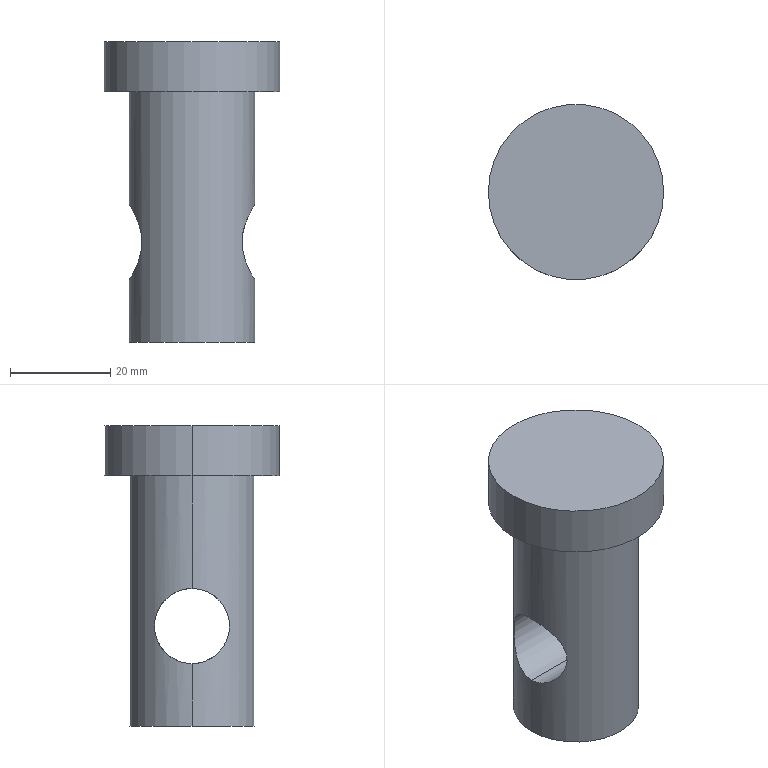Part | SolidWorks | features ICE 2, Chamfer 1, Extrusion 1 | 1 solid | 9 faces | box 35 x 35 x 60 mm | volume 29956 mm3 | cylinder 6 | plane 3 | commonest cylinder face diameters 15 x2 25 x2 35 x2
STEP:
#1=CARTESIAN_POINT('',(-12.5,0.,27.5));
#2=VERTEX_POINT('',#1);
#3=CARTESIAN_POINT('',(-12.5,0.,12.5));
#4=VERTEX_POINT('',#3);
#5=CARTESIAN_POINT('',(-12.5,0.,27.5));
#6=CARTESIAN_POINT('',(-12.5,-0.5065,27.5));
#7=CARTESIAN_POINT('',(-12.469,-1.005,27.449));
#8=CARTESIAN_POINT('',(-12.381,-1.74,27.3));
#9=CARTESIAN_POINT('',(-12.344,-1.984,27.237));
#10=CARTESIAN_POINT('',(-12.258,-2.461,27.089));
#11=CARTESIAN_POINT('',(-12.209,-2.693,27.004));
#12=CARTESIAN_POINT('',(-12.1,-3.145,26.813));
#13=CARTESIAN_POINT('',(-12.041,-3.365,26.707));
#14=CARTESIAN_POINT('',(-11.912,-3.794,26.474));
#15=CARTESIAN_POINT('',(-11.843,-4.004,26.347));
#16=CARTESIAN_POINT('',(-11.628,-4.606,25.939));
#17=CARTESIAN_POINT('',(-11.474,-4.974,25.633));
#18=CARTESIAN_POINT('',(-11.157,-5.65,24.956));
#19=CARTESIAN_POINT('',(-10.993,-5.957,24.581));
#20=CARTESIAN_POINT('',(-10.687,-6.49,23.788));
#21=CARTESIAN_POINT('',(-10.543,-6.72,23.367));
#22=CARTESIAN_POINT('',(-10.354,-7.005,22.691));
#23=CARTESIAN_POINT('',(-10.295,-7.09,22.458));
#24=CARTESIAN_POINT('',(-10.193,-7.237,21.985));
#25=CARTESIAN_POINT('',(-10.148,-7.298,21.745));
#26=CARTESIAN_POINT('',(-10.076,-7.398,21.258));
#27=CARTESIAN_POINT('',(-10.048,-7.436,21.011));
#28=CARTESIAN_POINT('',(-10.01,-7.487,20.509));
#29=CARTESIAN_POINT('',(-10.,-7.5,20.253));
#30=CARTESIAN_POINT('',(-10.,-7.5,19.498));
#31=CARTESIAN_POINT('',(-10.038,-7.45,19.));
#32=CARTESIAN_POINT('',(-10.147,-7.3,18.261));
#33=CARTESIAN_POINT('',(-10.192,-7.238,18.019));
#34=CARTESIAN_POINT('',(-10.294,-7.092,17.547));
#35=CARTESIAN_POINT('',(-10.352,-7.008,17.316));
#36=CARTESIAN_POINT('',(-10.54,-6.724,16.641));
#37=CARTESIAN_POINT('',(-10.688,-6.49,16.21));
#38=CARTESIAN_POINT('',(-10.995,-5.954,15.414));
#39=CARTESIAN_POINT('',(-11.156,-5.651,15.045));
#40=CARTESIAN_POINT('',(-11.476,-4.97,14.362));
#41=CARTESIAN_POINT('',(-11.63,-4.601,14.057));
#42=CARTESIAN_POINT('',(-11.843,-4.004,13.654));
#43=CARTESIAN_POINT('',(-11.911,-3.798,13.528));
#44=CARTESIAN_POINT('',(-12.039,-3.369,13.295));
#45=CARTESIAN_POINT('',(-12.1,-3.146,13.187));
#46=CARTESIAN_POINT('',(-12.264,-2.463,12.899));
#47=CARTESIAN_POINT('',(-12.35,-1.993,12.752));
#48=CARTESIAN_POINT('',(-12.439,-1.262,12.603));
#49=CARTESIAN_POINT('',(-12.461,-1.014,12.565));
#50=CARTESIAN_POINT('',(-12.492,-0.5103,12.513));
#51=CARTESIAN_POINT('',(-12.5,-0.2541,12.5));
#52=CARTESIAN_POINT('',(-12.5,0.,12.5));
#53=B_SPLINE_CURVE_WITH_KNOTS('',3,(#5,#6,#7,#8,#9,#10,#11,#12,#13,#14,#15,#16,#17,#18,#19,#20,#21,#22,#23,#24,#25,#26,#27,#28,#29,#30,#31,#32,#33,#34,#35,#36,#37,#38,#39,#40,#41,#42,#43,#44,#45,#46,#47,#48,#49,#50,#51,#52),.UNSPECIFIED.,.F.,.F.,(4,2,2,2,2,2,2,2,2,2,2,2,2,2,2,2,2,2,2,2,2,2,2,4),(0.02406,0.02556,0.02631,0.02706,0.02781,0.02856,0.03007,0.03157,0.03307,0.03382,0.03457,0.03532,0.03607,0.03757,0.03832,0.03907,0.04057,0.04207,0.04357,0.04432,0.04507,0.04658,0.04733,0.04808),.UNSPECIFIED.);
#54=EDGE_CURVE('',#2,#4,#53,.T.);
#55=ORIENTED_EDGE('',*,*,#54,.F.);
#56=CARTESIAN_POINT('',(12.5,0.,27.5));
#57=VERTEX_POINT('',#56);
#58=CARTESIAN_POINT('',(-30.,0.,27.5));
#59=DIRECTION('',(1.,0.,0.));
#60=VECTOR('',#59,1000.);
#61=LINE('',#58,#60);
#62=EDGE_CURVE('',#2,#57,#61,.T.);
#63=ORIENTED_EDGE('',*,*,#62,.T.);
#64=CARTESIAN_POINT('',(12.5,0.,12.5));
#65=VERTEX_POINT('',#64);
#66=CARTESIAN_POINT('',(12.5,0.,12.5));
#67=CARTESIAN_POINT('',(12.5,-0.5093,12.5));
#68=CARTESIAN_POINT('',(12.469,-1.008,12.551));
#69=CARTESIAN_POINT('',(12.351,-1.985,12.75));
#70=CARTESIAN_POINT('',(12.263,-2.468,12.901));
#71=CARTESIAN_POINT('',(12.045,-3.373,13.283));
#72=CARTESIAN_POINT('',(11.916,-3.8,13.516));
#73=CARTESIAN_POINT('',(11.628,-4.606,14.061));
#74=CARTESIAN_POINT('',(11.473,-4.976,14.368));
#75=CARTESIAN_POINT('',(11.236,-5.481,14.875));
#76=CARTESIAN_POINT('',(11.156,-5.641,15.052));
#77=CARTESIAN_POINT('',(10.996,-5.946,15.423));
#78=CARTESIAN_POINT('',(10.917,-6.091,15.617));
#79=CARTESIAN_POINT('',(10.686,-6.492,16.214));
#80=CARTESIAN_POINT('',(10.542,-6.721,16.636));
#81=CARTESIAN_POINT('',(10.291,-7.099,17.531));
#82=CARTESIAN_POINT('',(10.184,-7.249,18.011));
#83=CARTESIAN_POINT('',(10.076,-7.398,18.743));
#84=CARTESIAN_POINT('',(10.048,-7.436,18.989));
#85=CARTESIAN_POINT('',(10.01,-7.487,19.489));
#86=CARTESIAN_POINT('',(10.,-7.5,19.743));
#87=CARTESIAN_POINT('',(10.,-7.5,20.505));
#88=CARTESIAN_POINT('',(10.039,-7.449,21.004));
#89=CARTESIAN_POINT('',(10.147,-7.3,21.738));
#90=CARTESIAN_POINT('',(10.192,-7.238,21.982));
#91=CARTESIAN_POINT('',(10.294,-7.091,22.456));
#92=CARTESIAN_POINT('',(10.352,-7.007,22.686));
#93=CARTESIAN_POINT('',(10.478,-6.817,23.136));
#94=CARTESIAN_POINT('',(10.546,-6.712,23.355));
#95=CARTESIAN_POINT('',(10.69,-6.481,23.782));
#96=CARTESIAN_POINT('',(10.765,-6.355,23.991));
#97=CARTESIAN_POINT('',(10.997,-5.952,24.589));
#98=CARTESIAN_POINT('',(11.157,-5.649,24.957));
#99=CARTESIAN_POINT('',(11.396,-5.141,25.467));
#100=CARTESIAN_POINT('',(11.475,-4.961,25.63));
#101=CARTESIAN_POINT('',(11.629,-4.59,25.936));
#102=CARTESIAN_POINT('',(11.703,-4.397,26.08));
#103=CARTESIAN_POINT('',(11.916,-3.8,26.484));
#104=CARTESIAN_POINT('',(12.045,-3.375,26.716));
#105=CARTESIAN_POINT('',(12.209,-2.691,27.005));
#106=CARTESIAN_POINT('',(12.259,-2.456,27.091));
#107=CARTESIAN_POINT('',(12.344,-1.982,27.238));
#108=CARTESIAN_POINT('',(12.38,-1.742,27.299));
#109=CARTESIAN_POINT('',(12.439,-1.255,27.398));
#110=CARTESIAN_POINT('',(12.462,-1.009,27.436));
#111=CARTESIAN_POINT('',(12.492,-0.5089,27.487));
#112=CARTESIAN_POINT('',(12.5,-0.2538,27.5));
#113=CARTESIAN_POINT('',(12.5,0.,27.5));
#114=B_SPLINE_CURVE_WITH_KNOTS('',3,(#66,#67,#68,#69,#70,#71,#72,#73,#74,#75,#76,#77,#78,#79,#80,#81,#82,#83,#84,#85,#86,#87,#88,#89,#90,#91,#92,#93,#94,#95,#96,#97,#98,#99,#100,#101,#102,#103,#104,#105,#106,#107,#108,#109,#110,#111,#112,#113),.UNSPECIFIED.,.F.,.F.,(4,2,2,2,2,2,2,2,2,2,2,2,2,2,2,2,2,2,2,2,2,2,2,4),(0.,0.001504,0.003008,0.004512,0.006015,0.006767,0.007519,0.009023,0.01053,0.01128,0.01203,0.01353,0.01429,0.01504,0.01579,0.01654,0.01805,0.0188,0.01955,0.02105,0.02181,0.02256,0.02331,0.02406),.UNSPECIFIED.);
#115=EDGE_CURVE('',#65,#57,#114,.T.);
#116=ORIENTED_EDGE('',*,*,#115,.F.);
#117=CARTESIAN_POINT('',(-30.,0.,12.5));
#118=DIRECTION('',(1.,0.,0.));
#119=VECTOR('',#118,1000.);
#120=LINE('',#117,#119);
#121=EDGE_CURVE('',#4,#65,#120,.T.);
#122=ORIENTED_EDGE('',*,*,#121,.F.);
#123=EDGE_LOOP('',(#55,#63,#116,#122));
#124=FACE_OUTER_BOUND('',#123,.T.);
#125=CARTESIAN_POINT('',(-30.,0.,20.));
#126=DIRECTION('',(1.,0.,0.));
#127=DIRECTION('',(0.,0.,-1.));
#128=AXIS2_PLACEMENT_3D('',#125,#126,#127);
#129=CYLINDRICAL_SURFACE('',#128,7.5);
#130=ADVANCED_FACE('',(#124),#129,.F.);
#131=CARTESIAN_POINT('',(-12.5,0.,50.));
#132=VERTEX_POINT('',#131);
#133=CARTESIAN_POINT('',(12.5,0.,50.));
#134=VERTEX_POINT('',#133);
#135=CARTESIAN_POINT('',(0.,0.,50.));
#136=DIRECTION('',(0.,0.,-1.));
#137=DIRECTION('',(-1.,0.,0.));
#138=AXIS2_PLACEMENT_3D('',#135,#136,#137);
#139=CIRCLE('',#138,12.5);
#140=EDGE_CURVE('',#132,#134,#139,.T.);
#141=ORIENTED_EDGE('',*,*,#140,.T.);
#142=CARTESIAN_POINT('',(12.5,0.,50.));
#143=DIRECTION('',(0.,0.,-1.));
#144=VECTOR('',#143,1000.);
#145=LINE('',#142,#144);
#146=EDGE_CURVE('',#134,#57,#145,.T.);
#147=ORIENTED_EDGE('',*,*,#146,.T.);
#148=CARTESIAN_POINT('',(12.5,0.,27.5));
#149=CARTESIAN_POINT('',(12.5,0.5065,27.5));
#150=CARTESIAN_POINT('',(12.469,1.005,27.449));
#151=CARTESIAN_POINT('',(12.381,1.74,27.3));
#152=CARTESIAN_POINT('',(12.344,1.984,27.237));
#153=CARTESIAN_POINT('',(12.258,2.461,27.089));
#154=CARTESIAN_POINT('',(12.209,2.693,27.004));
#155=CARTESIAN_POINT('',(12.1,3.145,26.813));
#156=CARTESIAN_POINT('',(12.041,3.365,26.707));
#157=CARTESIAN_POINT('',(11.912,3.794,26.474));
#158=CARTESIAN_POINT('',(11.843,4.004,26.347));
#159=CARTESIAN_POINT('',(11.628,4.606,25.939));
#160=CARTESIAN_POINT('',(11.474,4.974,25.633));
#161=CARTESIAN_POINT('',(11.157,5.65,24.956));
#162=CARTESIAN_POINT('',(10.993,5.957,24.581));
#163=CARTESIAN_POINT('',(10.687,6.49,23.788));
#164=CARTESIAN_POINT('',(10.543,6.72,23.367));
#165=CARTESIAN_POINT('',(10.354,7.005,22.691));
#166=CARTESIAN_POINT('',(10.295,7.09,22.458));
#167=CARTESIAN_POINT('',(10.193,7.237,21.985));
#168=CARTESIAN_POINT('',(10.148,7.298,21.745));
#169=CARTESIAN_POINT('',(10.076,7.398,21.258));
#170=CARTESIAN_POINT('',(10.048,7.436,21.011));
#171=CARTESIAN_POINT('',(10.01,7.487,20.509));
#172=CARTESIAN_POINT('',(10.,7.5,20.253));
#173=CARTESIAN_POINT('',(10.,7.5,19.498));
#174=CARTESIAN_POINT('',(10.038,7.45,19.));
#175=CARTESIAN_POINT('',(10.147,7.3,18.261));
#176=CARTESIAN_POINT('',(10.192,7.238,18.019));
#177=CARTESIAN_POINT('',(10.294,7.092,17.547));
#178=CARTESIAN_POINT('',(10.352,7.008,17.316));
#179=CARTESIAN_POINT('',(10.54,6.724,16.641));
#180=CARTESIAN_POINT('',(10.688,6.49,16.21));
#181=CARTESIAN_POINT('',(10.995,5.954,15.414));
#182=CARTESIAN_POINT('',(11.156,5.651,15.045));
#183=CARTESIAN_POINT('',(11.476,4.97,14.362));
#184=CARTESIAN_POINT('',(11.63,4.601,14.057));
#185=CARTESIAN_POINT('',(11.843,4.004,13.654));
#186=CARTESIAN_POINT('',(11.911,3.798,13.528));
#187=CARTESIAN_POINT('',(12.039,3.369,13.295));
#188=CARTESIAN_POINT('',(12.1,3.146,13.187));
#189=CARTESIAN_POINT('',(12.264,2.463,12.899));
#190=CARTESIAN_POINT('',(12.35,1.993,12.752));
#191=CARTESIAN_POINT('',(12.439,1.262,12.603));
#192=CARTESIAN_POINT('',(12.461,1.014,12.565));
#193=CARTESIAN_POINT('',(12.492,0.5103,12.513));
#194=CARTESIAN_POINT('',(12.5,0.2541,12.5));
#195=CARTESIAN_POINT('',(12.5,0.,12.5));
#196=B_SPLINE_CURVE_WITH_KNOTS('',3,(#148,#149,#150,#151,#152,#153,#154,#155,#156,#157,#158,#159,#160,#161,#162,#163,#164,#165,#166,#167,#168,#169,#170,#171,#172,#173,#174,#175,#176,#177,#178,#179,#180,#181,#182,#183,#184,#185,#186,#187,#188,#189,#190,#191,#192,#193,#194,#195),.UNSPECIFIED.,.F.,.F.,(4,2,2,2,2,2,2,2,2,2,2,2,2,2,2,2,2,2,2,2,2,2,2,4),(0.02406,0.02556,0.02631,0.02706,0.02781,0.02856,0.03007,0.03157,0.03307,0.03382,0.03457,0.03532,0.03607,0.03757,0.03832,0.03907,0.04057,0.04207,0.04357,0.04432,0.04507,0.04658,0.04733,0.04808),.UNSPECIFIED.);
#197=EDGE_CURVE('',#57,#65,#196,.T.);
#198=ORIENTED_EDGE('',*,*,#197,.T.);
#199=CARTESIAN_POINT('',(12.5,0.,0.));
#200=VERTEX_POINT('',#199);
#201=CARTESIAN_POINT('',(12.5,0.,50.));
#202=DIRECTION('',(0.,0.,-1.));
#203=VECTOR('',#202,1000.);
#204=LINE('',#201,#203);
#205=EDGE_CURVE('',#65,#200,#204,.T.);
#206=ORIENTED_EDGE('',*,*,#205,.T.);
#207=CARTESIAN_POINT('',(-12.5,0.,0.));
#208=VERTEX_POINT('',#207);
#209=CARTESIAN_POINT('',(0.,0.,0.));
#210=DIRECTION('',(0.,0.,-1.));
#211=DIRECTION('',(-1.,0.,0.));
#212=AXIS2_PLACEMENT_3D('',#209,#210,#211);
#213=CIRCLE('',#212,12.5);
#214=EDGE_CURVE('',#208,#200,#213,.T.);
#215=ORIENTED_EDGE('',*,*,#214,.F.);
#216=CARTESIAN_POINT('',(-12.5,0.,50.));
#217=DIRECTION('',(0.,0.,-1.));
#218=VECTOR('',#217,1000.);
#219=LINE('',#216,#218);
#220=EDGE_CURVE('',#4,#208,#219,.T.);
#221=ORIENTED_EDGE('',*,*,#220,.F.);
#222=CARTESIAN_POINT('',(-12.5,0.,12.5));
#223=CARTESIAN_POINT('',(-12.5,0.5093,12.5));
#224=CARTESIAN_POINT('',(-12.469,1.008,12.551));
#225=CARTESIAN_POINT('',(-12.351,1.985,12.75));
#226=CARTESIAN_POINT('',(-12.263,2.468,12.901));
#227=CARTESIAN_POINT('',(-12.045,3.373,13.283));
#228=CARTESIAN_POINT('',(-11.916,3.8,13.516));
#229=CARTESIAN_POINT('',(-11.628,4.606,14.061));
#230=CARTESIAN_POINT('',(-11.473,4.976,14.368));
#231=CARTESIAN_POINT('',(-11.236,5.481,14.875));
#232=CARTESIAN_POINT('',(-11.156,5.641,15.052));
#233=CARTESIAN_POINT('',(-10.996,5.946,15.423));
#234=CARTESIAN_POINT('',(-10.917,6.091,15.617));
#235=CARTESIAN_POINT('',(-10.686,6.492,16.214));
#236=CARTESIAN_POINT('',(-10.542,6.721,16.636));
#237=CARTESIAN_POINT('',(-10.291,7.099,17.531));
#238=CARTESIAN_POINT('',(-10.184,7.249,18.011));
#239=CARTESIAN_POINT('',(-10.076,7.398,18.743));
#240=CARTESIAN_POINT('',(-10.048,7.436,18.989));
#241=CARTESIAN_POINT('',(-10.01,7.487,19.489));
#242=CARTESIAN_POINT('',(-10.,7.5,19.743));
#243=CARTESIAN_POINT('',(-10.,7.5,20.505));
#244=CARTESIAN_POINT('',(-10.039,7.449,21.004));
#245=CARTESIAN_POINT('',(-10.147,7.3,21.738));
#246=CARTESIAN_POINT('',(-10.192,7.238,21.982));
#247=CARTESIAN_POINT('',(-10.294,7.091,22.456));
#248=CARTESIAN_POINT('',(-10.352,7.007,22.686));
#249=CARTESIAN_POINT('',(-10.478,6.817,23.136));
#250=CARTESIAN_POINT('',(-10.546,6.712,23.355));
#251=CARTESIAN_POINT('',(-10.69,6.481,23.782));
#252=CARTESIAN_POINT('',(-10.765,6.355,23.991));
#253=CARTESIAN_POINT('',(-10.997,5.952,24.589));
#254=CARTESIAN_POINT('',(-11.157,5.649,24.957));
#255=CARTESIAN_POINT('',(-11.396,5.141,25.467));
#256=CARTESIAN_POINT('',(-11.475,4.961,25.63));
#257=CARTESIAN_POINT('',(-11.629,4.59,25.936));
#258=CARTESIAN_POINT('',(-11.703,4.397,26.08));
#259=CARTESIAN_POINT('',(-11.916,3.8,26.484));
#260=CARTESIAN_POINT('',(-12.045,3.375,26.716));
#261=CARTESIAN_POINT('',(-12.209,2.691,27.005));
#262=CARTESIAN_POINT('',(-12.259,2.456,27.091));
#263=CARTESIAN_POINT('',(-12.344,1.982,27.238));
#264=CARTESIAN_POINT('',(-12.38,1.742,27.299));
#265=CARTESIAN_POINT('',(-12.439,1.255,27.398));
#266=CARTESIAN_POINT('',(-12.462,1.009,27.436));
#267=CARTESIAN_POINT('',(-12.492,0.5089,27.487));
#268=CARTESIAN_POINT('',(-12.5,0.2538,27.5));
#269=CARTESIAN_POINT('',(-12.5,0.,27.5));
#270=B_SPLINE_CURVE_WITH_KNOTS('',3,(#222,#223,#224,#225,#226,#227,#228,#229,#230,#231,#232,#233,#234,#235,#236,#237,#238,#239,#240,#241,#242,#243,#244,#245,#246,#247,#248,#249,#250,#251,#252,#253,#254,#255,#256,#257,#258,#259,#260,#261,#262,#263,#264,#265,#266,#267,#268,#269),.UNSPECIFIED.,.F.,.F.,(4,2,2,2,2,2,2,2,2,2,2,2,2,2,2,2,2,2,2,2,2,2,2,4),(0.,0.001504,0.003008,0.004512,0.006015,0.006767,0.007519,0.009023,0.01053,0.01128,0.01203,0.01353,0.01429,0.01504,0.01579,0.01654,0.01805,0.0188,0.01955,0.02105,0.02181,0.02256,0.02331,0.02406),.UNSPECIFIED.);
#271=EDGE_CURVE('',#4,#2,#270,.T.);
#272=ORIENTED_EDGE('',*,*,#271,.T.);
#273=CARTESIAN_POINT('',(-12.5,0.,50.));
#274=DIRECTION('',(0.,0.,-1.));
#275=VECTOR('',#274,1000.);
#276=LINE('',#273,#275);
#277=EDGE_CURVE('',#132,#2,#276,.T.);
#278=ORIENTED_EDGE('',*,*,#277,.F.);
#279=EDGE_LOOP('',(#141,#147,#198,#206,#215,#221,#272,#278));
#280=FACE_OUTER_BOUND('',#279,.T.);
#281=CARTESIAN_POINT('',(0.,0.,50.));
#282=DIRECTION('',(0.,0.,-1.));
#283=DIRECTION('',(-1.,0.,0.));
#284=AXIS2_PLACEMENT_3D('',#281,#282,#283);
#285=CYLINDRICAL_SURFACE('',#284,12.5);
#286=ADVANCED_FACE('',(#280),#285,.T.);
#287=CARTESIAN_POINT('',(17.5,0.,60.));
#288=VERTEX_POINT('',#287);
#289=CARTESIAN_POINT('',(-17.5,0.,60.));
#290=VERTEX_POINT('',#289);
#291=CARTESIAN_POINT('',(0.,0.,60.));
#292=DIRECTION('',(0.,0.,1.));
#293=DIRECTION('',(1.,0.,0.));
#294=AXIS2_PLACEMENT_3D('',#291,#292,#293);
#295=CIRCLE('',#294,17.5);
#296=EDGE_CURVE('',#288,#290,#295,.T.);
#297=ORIENTED_EDGE('',*,*,#296,.F.);
#298=CARTESIAN_POINT('',(17.5,0.,50.));
#299=VERTEX_POINT('',#298);
#300=CARTESIAN_POINT('',(17.5,0.,60.));
#301=DIRECTION('',(0.,0.,-1.));
#302=VECTOR('',#301,1000.);
#303=LINE('',#300,#302);
#304=EDGE_CURVE('',#288,#299,#303,.T.);
#305=ORIENTED_EDGE('',*,*,#304,.T.);
#306=CARTESIAN_POINT('',(-17.5,0.,50.));
#307=VERTEX_POINT('',#306);
#308=CARTESIAN_POINT('',(0.,0.,50.));
#309=DIRECTION('',(0.,0.,-1.));
#310=DIRECTION('',(-1.,0.,0.));
#311=AXIS2_PLACEMENT_3D('',#308,#309,#310);
#312=CIRCLE('',#311,17.5);
#313=EDGE_CURVE('',#307,#299,#312,.T.);
#314=ORIENTED_EDGE('',*,*,#313,.F.);
#315=CARTESIAN_POINT('',(-17.5,0.,60.));
#316=DIRECTION('',(0.,0.,-1.));
#317=VECTOR('',#316,1000.);
#318=LINE('',#315,#317);
#319=EDGE_CURVE('',#290,#307,#318,.T.);
#320=ORIENTED_EDGE('',*,*,#319,.F.);
#321=EDGE_LOOP('',(#297,#305,#314,#320));
#322=FACE_OUTER_BOUND('',#321,.T.);
#323=CARTESIAN_POINT('',(0.,0.,60.));
#324=DIRECTION('',(0.,0.,-1.));
#325=DIRECTION('',(-1.,0.,0.));
#326=AXIS2_PLACEMENT_3D('',#323,#324,#325);
#327=CYLINDRICAL_SURFACE('',#326,17.5);
#328=ADVANCED_FACE('',(#322),#327,.T.);
#329=ORIENTED_EDGE('',*,*,#304,.F.);
#330=CARTESIAN_POINT('',(0.,0.,60.));
#331=DIRECTION('',(0.,0.,1.));
#332=DIRECTION('',(1.,0.,0.));
#333=AXIS2_PLACEMENT_3D('',#330,#331,#332);
#334=CIRCLE('',#333,17.5);
#335=EDGE_CURVE('',#290,#288,#334,.T.);
#336=ORIENTED_EDGE('',*,*,#335,.F.);
#337=ORIENTED_EDGE('',*,*,#319,.T.);
#338=CARTESIAN_POINT('',(0.,0.,50.));
#339=DIRECTION('',(0.,0.,-1.));
#340=DIRECTION('',(-1.,0.,0.));
#341=AXIS2_PLACEMENT_3D('',#338,#339,#340);
#342=CIRCLE('',#341,17.5);
#343=EDGE_CURVE('',#299,#307,#342,.T.);
#344=ORIENTED_EDGE('',*,*,#343,.F.);
#345=EDGE_LOOP('',(#329,#336,#337,#344));
#346=FACE_OUTER_BOUND('',#345,.T.);
#347=CARTESIAN_POINT('',(0.,0.,60.));
#348=DIRECTION('',(0.,0.,-1.));
#349=DIRECTION('',(-1.,0.,0.));
#350=AXIS2_PLACEMENT_3D('',#347,#348,#349);
#351=CYLINDRICAL_SURFACE('',#350,17.5);
#352=ADVANCED_FACE('',(#346),#351,.T.);
#353=ORIENTED_EDGE('',*,*,#335,.T.);
#354=ORIENTED_EDGE('',*,*,#296,.T.);
#355=EDGE_LOOP('',(#353,#354));
#356=FACE_OUTER_BOUND('',#355,.T.);
#357=CARTESIAN_POINT('',(0.,0.,60.));
#358=DIRECTION('',(0.,0.,1.));
#359=DIRECTION('',(1.,0.,0.));
#360=AXIS2_PLACEMENT_3D('',#357,#358,#359);
#361=PLANE('',#360);
#362=ADVANCED_FACE('',(#356),#361,.T.);
#363=ORIENTED_EDGE('',*,*,#140,.F.);
#364=CARTESIAN_POINT('',(0.,0.,50.));
#365=DIRECTION('',(0.,0.,-1.));
#366=DIRECTION('',(-1.,0.,0.));
#367=AXIS2_PLACEMENT_3D('',#364,#365,#366);
#368=CIRCLE('',#367,12.5);
#369=EDGE_CURVE('',#134,#132,#368,.T.);
#370=ORIENTED_EDGE('',*,*,#369,.F.);
#371=EDGE_LOOP('',(#363,#370));
#372=FACE_BOUND('',#371,.T.);
#373=ORIENTED_EDGE('',*,*,#313,.T.);
#374=ORIENTED_EDGE('',*,*,#343,.T.);
#375=EDGE_LOOP('',(#373,#374));
#376=FACE_OUTER_BOUND('',#375,.T.);
#377=CARTESIAN_POINT('',(0.,0.,50.));
#378=DIRECTION('',(0.,0.,-1.));
#379=DIRECTION('',(-1.,0.,0.));
#380=AXIS2_PLACEMENT_3D('',#377,#378,#379);
#381=PLANE('',#380);
#382=ADVANCED_FACE('',(#372,#376),#381,.T.);
#383=ORIENTED_EDGE('',*,*,#146,.F.);
#384=ORIENTED_EDGE('',*,*,#369,.T.);
#385=ORIENTED_EDGE('',*,*,#277,.T.);
#386=ORIENTED_EDGE('',*,*,#54,.T.);
#387=ORIENTED_EDGE('',*,*,#220,.T.);
#388=CARTESIAN_POINT('',(0.,0.,0.));
#389=DIRECTION('',(0.,0.,-1.));
#390=DIRECTION('',(-1.,0.,0.));
#391=AXIS2_PLACEMENT_3D('',#388,#389,#390);
#392=CIRCLE('',#391,12.5);
#393=EDGE_CURVE('',#200,#208,#392,.T.);
#394=ORIENTED_EDGE('',*,*,#393,.F.);
#395=ORIENTED_EDGE('',*,*,#205,.F.);
#396=ORIENTED_EDGE('',*,*,#115,.T.);
#397=EDGE_LOOP('',(#383,#384,#385,#386,#387,#394,#395,#396));
#398=FACE_OUTER_BOUND('',#397,.T.);
#399=CARTESIAN_POINT('',(0.,0.,50.));
#400=DIRECTION('',(0.,0.,-1.));
#401=DIRECTION('',(-1.,0.,0.));
#402=AXIS2_PLACEMENT_3D('',#399,#400,#401);
#403=CYLINDRICAL_SURFACE('',#402,12.5);
#404=ADVANCED_FACE('',(#398),#403,.T.);
#405=ORIENTED_EDGE('',*,*,#214,.T.);
#406=ORIENTED_EDGE('',*,*,#393,.T.);
#407=EDGE_LOOP('',(#405,#406));
#408=FACE_OUTER_BOUND('',#407,.T.);
#409=CARTESIAN_POINT('',(0.,0.,0.));
#410=DIRECTION('',(0.,0.,1.));
#411=DIRECTION('',(1.,0.,0.));
#412=AXIS2_PLACEMENT_3D('',#409,#410,#411);
#413=PLANE('',#412);
#414=ADVANCED_FACE('',(#408),#413,.F.);
#415=ORIENTED_EDGE('',*,*,#62,.F.);
#416=ORIENTED_EDGE('',*,*,#271,.F.);
#417=ORIENTED_EDGE('',*,*,#121,.T.);
#418=ORIENTED_EDGE('',*,*,#197,.F.);
#419=EDGE_LOOP('',(#415,#416,#417,#418));
#420=FACE_OUTER_BOUND('',#419,.T.);
#421=CARTESIAN_POINT('',(-30.,0.,20.));
#422=DIRECTION('',(1.,0.,0.));
#423=DIRECTION('',(0.,0.,-1.));
#424=AXIS2_PLACEMENT_3D('',#421,#422,#423);
#425=CYLINDRICAL_SURFACE('',#424,7.5);
#426=ADVANCED_FACE('',(#420),#425,.F.);
#427=CLOSED_SHELL('',(#130,#286,#328,#352,#362,#382,#404,#414,#426));
#428=MANIFOLD_SOLID_BREP('',#427);
#429=CARTESIAN_POINT('',(0.,0.,0.));
#430=DIRECTION('',(0.,0.,1.));
#431=DIRECTION('',(1.,0.,0.));
#432=AXIS2_PLACEMENT_3D('',#429,#430,#431);
#433=(LENGTH_UNIT()NAMED_UNIT(*)SI_UNIT(.MILLI.,.METRE.));
#434=UNCERTAINTY_MEASURE_WITH_UNIT(LENGTH_MEASURE(0.00001),#433,'','');
#435=(NAMED_UNIT(*)PLANE_ANGLE_UNIT()SI_UNIT($,.RADIAN.));
#436=(NAMED_UNIT(*)SI_UNIT($,.STERADIAN.)SOLID_ANGLE_UNIT());
#437=(GEOMETRIC_REPRESENTATION_CONTEXT(3)GLOBAL_UNCERTAINTY_ASSIGNED_CONTEXT((#434))GLOBAL_UNIT_ASSIGNED_CONTEXT((#433,#435,#436))REPRESENTATION_CONTEXT('',''));
#438=ADVANCED_BREP_SHAPE_REPRESENTATION('',(#428,#432),#437);